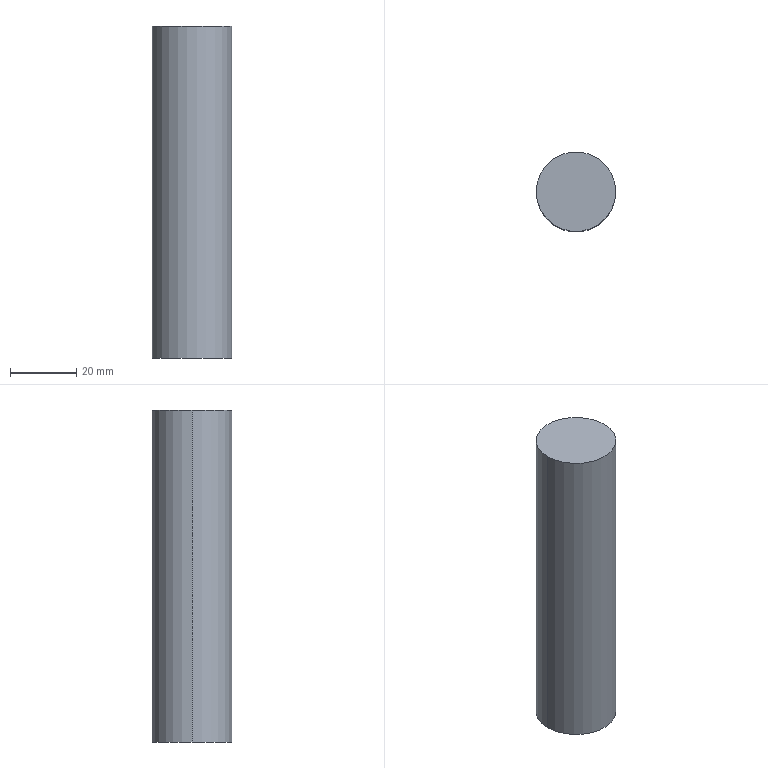Part | SolidWorks | features Extrusion 1 | 1 solid | 4 faces | box 24 x 24 x 100 mm | volume 45239 mm3 | cylinder 2 | plane 2 | commonest cylinder face diameters 24 x2
STEP:
#1=CARTESIAN_POINT('',(12.,0.,100.));
#2=VERTEX_POINT('',#1);
#3=CARTESIAN_POINT('',(-12.,0.,100.));
#4=VERTEX_POINT('',#3);
#5=CARTESIAN_POINT('',(0.,0.,100.));
#6=DIRECTION('',(0.,0.,1.));
#7=DIRECTION('',(1.,0.,0.));
#8=AXIS2_PLACEMENT_3D('',#5,#6,#7);
#9=CIRCLE('',#8,12.);
#10=EDGE_CURVE('',#2,#4,#9,.T.);
#11=ORIENTED_EDGE('',*,*,#10,.F.);
#12=CARTESIAN_POINT('',(12.,0.,0.));
#13=VERTEX_POINT('',#12);
#14=CARTESIAN_POINT('',(12.,0.,100.));
#15=DIRECTION('',(0.,0.,-1.));
#16=VECTOR('',#15,1000.);
#17=LINE('',#14,#16);
#18=EDGE_CURVE('',#2,#13,#17,.T.);
#19=ORIENTED_EDGE('',*,*,#18,.T.);
#20=CARTESIAN_POINT('',(-12.,0.,0.));
#21=VERTEX_POINT('',#20);
#22=CARTESIAN_POINT('',(0.,0.,0.));
#23=DIRECTION('',(0.,0.,1.));
#24=DIRECTION('',(1.,0.,0.));
#25=AXIS2_PLACEMENT_3D('',#22,#23,#24);
#26=CIRCLE('',#25,12.);
#27=EDGE_CURVE('',#13,#21,#26,.T.);
#28=ORIENTED_EDGE('',*,*,#27,.T.);
#29=CARTESIAN_POINT('',(-12.,0.,100.));
#30=DIRECTION('',(0.,0.,-1.));
#31=VECTOR('',#30,1000.);
#32=LINE('',#29,#31);
#33=EDGE_CURVE('',#4,#21,#32,.T.);
#34=ORIENTED_EDGE('',*,*,#33,.F.);
#35=EDGE_LOOP('',(#11,#19,#28,#34));
#36=FACE_OUTER_BOUND('',#35,.T.);
#37=CARTESIAN_POINT('',(0.,0.,100.));
#38=DIRECTION('',(0.,0.,-1.));
#39=DIRECTION('',(-1.,0.,0.));
#40=AXIS2_PLACEMENT_3D('',#37,#38,#39);
#41=CYLINDRICAL_SURFACE('',#40,12.);
#42=ADVANCED_FACE('',(#36),#41,.T.);
#43=ORIENTED_EDGE('',*,*,#18,.F.);
#44=CARTESIAN_POINT('',(0.,0.,100.));
#45=DIRECTION('',(0.,0.,1.));
#46=DIRECTION('',(1.,0.,0.));
#47=AXIS2_PLACEMENT_3D('',#44,#45,#46);
#48=CIRCLE('',#47,12.);
#49=EDGE_CURVE('',#4,#2,#48,.T.);
#50=ORIENTED_EDGE('',*,*,#49,.F.);
#51=ORIENTED_EDGE('',*,*,#33,.T.);
#52=CARTESIAN_POINT('',(0.,0.,0.));
#53=DIRECTION('',(0.,0.,1.));
#54=DIRECTION('',(1.,0.,0.));
#55=AXIS2_PLACEMENT_3D('',#52,#53,#54);
#56=CIRCLE('',#55,12.);
#57=EDGE_CURVE('',#21,#13,#56,.T.);
#58=ORIENTED_EDGE('',*,*,#57,.T.);
#59=EDGE_LOOP('',(#43,#50,#51,#58));
#60=FACE_OUTER_BOUND('',#59,.T.);
#61=CARTESIAN_POINT('',(0.,0.,100.));
#62=DIRECTION('',(0.,0.,-1.));
#63=DIRECTION('',(-1.,0.,0.));
#64=AXIS2_PLACEMENT_3D('',#61,#62,#63);
#65=CYLINDRICAL_SURFACE('',#64,12.);
#66=ADVANCED_FACE('',(#60),#65,.T.);
#67=ORIENTED_EDGE('',*,*,#49,.T.);
#68=ORIENTED_EDGE('',*,*,#10,.T.);
#69=EDGE_LOOP('',(#67,#68));
#70=FACE_OUTER_BOUND('',#69,.T.);
#71=CARTESIAN_POINT('',(0.,0.,100.));
#72=DIRECTION('',(0.,0.,1.));
#73=DIRECTION('',(1.,0.,0.));
#74=AXIS2_PLACEMENT_3D('',#71,#72,#73);
#75=PLANE('',#74);
#76=ADVANCED_FACE('',(#70),#75,.T.);
#77=ORIENTED_EDGE('',*,*,#57,.F.);
#78=ORIENTED_EDGE('',*,*,#27,.F.);
#79=EDGE_LOOP('',(#77,#78));
#80=FACE_OUTER_BOUND('',#79,.T.);
#81=CARTESIAN_POINT('',(0.,0.,0.));
#82=DIRECTION('',(0.,0.,1.));
#83=DIRECTION('',(1.,0.,0.));
#84=AXIS2_PLACEMENT_3D('',#81,#82,#83);
#85=PLANE('',#84);
#86=ADVANCED_FACE('',(#80),#85,.F.);
#87=CLOSED_SHELL('',(#42,#66,#76,#86));
#88=MANIFOLD_SOLID_BREP('',#87);
#89=CARTESIAN_POINT('',(0.,0.,0.));
#90=DIRECTION('',(0.,0.,1.));
#91=DIRECTION('',(1.,0.,0.));
#92=AXIS2_PLACEMENT_3D('',#89,#90,#91);
#93=(LENGTH_UNIT()NAMED_UNIT(*)SI_UNIT(.MILLI.,.METRE.));
#94=UNCERTAINTY_MEASURE_WITH_UNIT(LENGTH_MEASURE(0.00001),#93,'','');
#95=(NAMED_UNIT(*)PLANE_ANGLE_UNIT()SI_UNIT($,.RADIAN.));
#96=(NAMED_UNIT(*)SI_UNIT($,.STERADIAN.)SOLID_ANGLE_UNIT());
#97=(GEOMETRIC_REPRESENTATION_CONTEXT(3)GLOBAL_UNCERTAINTY_ASSIGNED_CONTEXT((#94))GLOBAL_UNIT_ASSIGNED_CONTEXT((#93,#95,#96))REPRESENTATION_CONTEXT('',''));
#98=ADVANCED_BREP_SHAPE_REPRESENTATION('',(#88,#92),#97);